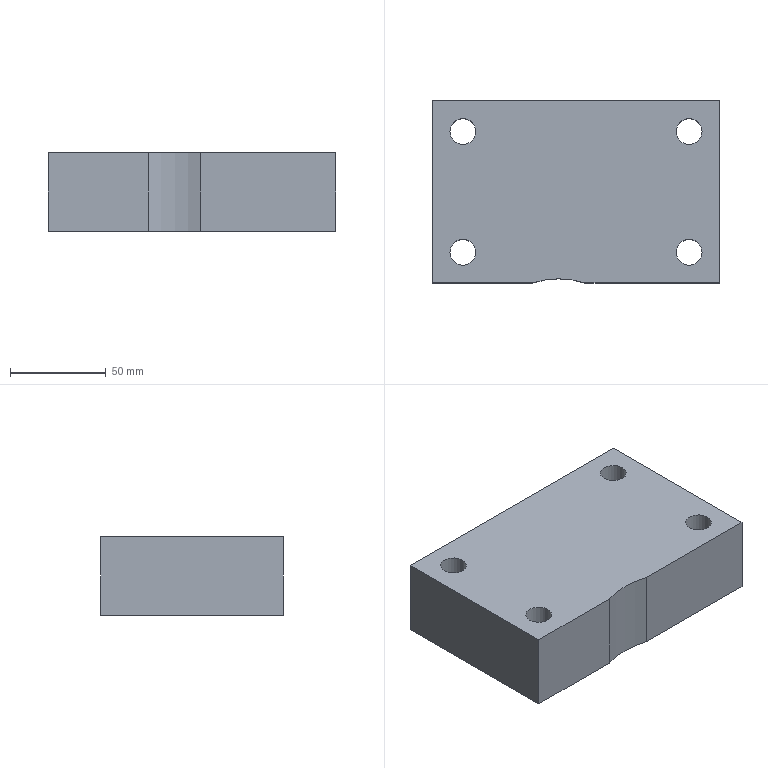Part | NX | features solid 2 | 1 solid | 20 faces | box 150 x 95 x 41 mm | volume 548863 mm3 | plane 11 | cylinder 9 | commonest cylinder face diameters 13.5 x4 20 x4 88 x1
STEP:
#1=CARTESIAN_POINT('',(1702.713,264.808,60.));
#2=VERTEX_POINT('',#1);
#3=CARTESIAN_POINT('',(1702.713,264.808,101.));
#4=VERTEX_POINT('',#3);
#5=CARTESIAN_POINT('',(1702.713,264.808,50.));
#6=DIRECTION('',(0.,0.,1.));
#7=VECTOR('',#6,1000.);
#8=LINE('',#5,#7);
#9=EDGE_CURVE('',#2,#4,#8,.T.);
#10=ORIENTED_EDGE('',*,*,#9,.F.);
#11=CARTESIAN_POINT('',(1773.045,264.808,60.));
#12=VERTEX_POINT('',#11);
#13=CARTESIAN_POINT('',(1698.045,264.808,60.));
#14=DIRECTION('',(1.,0.,0.));
#15=VECTOR('',#14,1000.);
#16=LINE('',#13,#15);
#17=EDGE_CURVE('',#2,#12,#16,.T.);
#18=ORIENTED_EDGE('',*,*,#17,.T.);
#19=CARTESIAN_POINT('',(1773.045,264.808,101.));
#20=VERTEX_POINT('',#19);
#21=CARTESIAN_POINT('',(1773.045,264.808,81.));
#22=DIRECTION('',(0.,0.,1.));
#23=VECTOR('',#22,1000.);
#24=LINE('',#21,#23);
#25=EDGE_CURVE('',#12,#20,#24,.T.);
#26=ORIENTED_EDGE('',*,*,#25,.T.);
#27=CARTESIAN_POINT('',(1698.045,264.808,101.));
#28=DIRECTION('',(-1.,0.,0.));
#29=VECTOR('',#28,1000.);
#30=LINE('',#27,#29);
#31=EDGE_CURVE('',#20,#4,#30,.T.);
#32=ORIENTED_EDGE('',*,*,#31,.T.);
#33=EDGE_LOOP('',(#10,#18,#26,#32));
#34=FACE_BOUND('',#33,.T.);
#35=CARTESIAN_POINT('',(1698.045,264.808,81.));
#36=DIRECTION('',(0.,-1.,0.));
#37=DIRECTION('',(0.,0.,1.));
#38=AXIS2_PLACEMENT_3D('',#35,#36,#37);
#39=PLANE('',#38);
#40=ADVANCED_FACE('',(#34),#39,.T.);
#41=CARTESIAN_POINT('',(1675.287,264.808,60.));
#42=VERTEX_POINT('',#41);
#43=CARTESIAN_POINT('',(1689.,223.,60.));
#44=DIRECTION('',(0.,0.,-1.));
#45=DIRECTION('',(-1.,0.,0.));
#46=AXIS2_PLACEMENT_3D('',#43,#44,#45);
#47=CIRCLE('',#46,44.);
#48=EDGE_CURVE('',#42,#2,#47,.T.);
#49=ORIENTED_EDGE('',*,*,#48,.F.);
#50=CARTESIAN_POINT('',(1623.045,264.808,60.));
#51=VERTEX_POINT('',#50);
#52=CARTESIAN_POINT('',(1698.045,264.808,60.));
#53=DIRECTION('',(1.,0.,0.));
#54=VECTOR('',#53,1000.);
#55=LINE('',#52,#54);
#56=EDGE_CURVE('',#51,#42,#55,.T.);
#57=ORIENTED_EDGE('',*,*,#56,.F.);
#58=CARTESIAN_POINT('',(1623.045,359.808,60.));
#59=VERTEX_POINT('',#58);
#60=CARTESIAN_POINT('',(1623.045,312.308,60.));
#61=DIRECTION('',(0.,-1.,0.));
#62=VECTOR('',#61,1000.);
#63=LINE('',#60,#62);
#64=EDGE_CURVE('',#59,#51,#63,.T.);
#65=ORIENTED_EDGE('',*,*,#64,.F.);
#66=CARTESIAN_POINT('',(1773.045,359.808,60.));
#67=VERTEX_POINT('',#66);
#68=CARTESIAN_POINT('',(1698.045,359.808,60.));
#69=DIRECTION('',(-1.,0.,0.));
#70=VECTOR('',#69,1000.);
#71=LINE('',#68,#70);
#72=EDGE_CURVE('',#67,#59,#71,.T.);
#73=ORIENTED_EDGE('',*,*,#72,.F.);
#74=CARTESIAN_POINT('',(1773.045,312.308,60.));
#75=DIRECTION('',(0.,1.,0.));
#76=VECTOR('',#75,1000.);
#77=LINE('',#74,#76);
#78=EDGE_CURVE('',#12,#67,#77,.T.);
#79=ORIENTED_EDGE('',*,*,#78,.F.);
#80=ORIENTED_EDGE('',*,*,#17,.F.);
#81=EDGE_LOOP('',(#49,#57,#65,#73,#79,#80));
#82=FACE_BOUND('',#81,.T.);
#83=CARTESIAN_POINT('',(1767.045,280.808,60.));
#84=VERTEX_POINT('',#83);
#85=CARTESIAN_POINT('',(1757.045,280.808,60.));
#86=DIRECTION('',(0.,0.,1.));
#87=DIRECTION('',(1.,0.,0.));
#88=AXIS2_PLACEMENT_3D('',#85,#86,#87);
#89=CIRCLE('',#88,10.);
#90=EDGE_CURVE('',#84,#84,#89,.T.);
#91=ORIENTED_EDGE('',*,*,#90,.T.);
#92=EDGE_LOOP('',(#91));
#93=FACE_BOUND('',#92,.T.);
#94=CARTESIAN_POINT('',(1649.045,343.808,60.));
#95=VERTEX_POINT('',#94);
#96=CARTESIAN_POINT('',(1639.045,343.808,60.));
#97=DIRECTION('',(0.,0.,1.));
#98=DIRECTION('',(1.,0.,0.));
#99=AXIS2_PLACEMENT_3D('',#96,#97,#98);
#100=CIRCLE('',#99,10.);
#101=EDGE_CURVE('',#95,#95,#100,.T.);
#102=ORIENTED_EDGE('',*,*,#101,.T.);
#103=EDGE_LOOP('',(#102));
#104=FACE_BOUND('',#103,.T.);
#105=CARTESIAN_POINT('',(1649.045,280.808,60.));
#106=VERTEX_POINT('',#105);
#107=CARTESIAN_POINT('',(1639.045,280.808,60.));
#108=DIRECTION('',(0.,0.,1.));
#109=DIRECTION('',(1.,0.,0.));
#110=AXIS2_PLACEMENT_3D('',#107,#108,#109);
#111=CIRCLE('',#110,10.);
#112=EDGE_CURVE('',#106,#106,#111,.T.);
#113=ORIENTED_EDGE('',*,*,#112,.T.);
#114=EDGE_LOOP('',(#113));
#115=FACE_BOUND('',#114,.T.);
#116=CARTESIAN_POINT('',(1767.045,343.808,60.));
#117=VERTEX_POINT('',#116);
#118=CARTESIAN_POINT('',(1757.045,343.808,60.));
#119=DIRECTION('',(0.,0.,1.));
#120=DIRECTION('',(1.,0.,0.));
#121=AXIS2_PLACEMENT_3D('',#118,#119,#120);
#122=CIRCLE('',#121,10.);
#123=EDGE_CURVE('',#117,#117,#122,.T.);
#124=ORIENTED_EDGE('',*,*,#123,.T.);
#125=EDGE_LOOP('',(#124));
#126=FACE_BOUND('',#125,.T.);
#127=CARTESIAN_POINT('',(1698.045,312.308,60.));
#128=DIRECTION('',(0.,0.,-1.));
#129=DIRECTION('',(1.,0.,0.));
#130=AXIS2_PLACEMENT_3D('',#127,#128,#129);
#131=PLANE('',#130);
#132=ADVANCED_FACE('',(#82,#93,#104,#115,#126),#131,.T.);
#133=CARTESIAN_POINT('',(1675.287,264.808,101.));
#134=VERTEX_POINT('',#133);
#135=CARTESIAN_POINT('',(1689.,223.,101.));
#136=DIRECTION('',(0.,0.,1.));
#137=DIRECTION('',(1.,0.,0.));
#138=AXIS2_PLACEMENT_3D('',#135,#136,#137);
#139=CIRCLE('',#138,44.);
#140=EDGE_CURVE('',#4,#134,#139,.T.);
#141=ORIENTED_EDGE('',*,*,#140,.F.);
#142=ORIENTED_EDGE('',*,*,#31,.F.);
#143=CARTESIAN_POINT('',(1773.045,359.808,101.));
#144=VERTEX_POINT('',#143);
#145=CARTESIAN_POINT('',(1773.045,312.308,101.));
#146=DIRECTION('',(0.,-1.,0.));
#147=VECTOR('',#146,1000.);
#148=LINE('',#145,#147);
#149=EDGE_CURVE('',#144,#20,#148,.T.);
#150=ORIENTED_EDGE('',*,*,#149,.F.);
#151=CARTESIAN_POINT('',(1623.045,359.808,101.));
#152=VERTEX_POINT('',#151);
#153=CARTESIAN_POINT('',(1698.045,359.808,101.));
#154=DIRECTION('',(1.,0.,0.));
#155=VECTOR('',#154,1000.);
#156=LINE('',#153,#155);
#157=EDGE_CURVE('',#152,#144,#156,.T.);
#158=ORIENTED_EDGE('',*,*,#157,.F.);
#159=CARTESIAN_POINT('',(1623.045,264.808,101.));
#160=VERTEX_POINT('',#159);
#161=CARTESIAN_POINT('',(1623.045,312.308,101.));
#162=DIRECTION('',(0.,1.,0.));
#163=VECTOR('',#162,1000.);
#164=LINE('',#161,#163);
#165=EDGE_CURVE('',#160,#152,#164,.T.);
#166=ORIENTED_EDGE('',*,*,#165,.F.);
#167=CARTESIAN_POINT('',(1698.045,264.808,101.));
#168=DIRECTION('',(-1.,0.,0.));
#169=VECTOR('',#168,1000.);
#170=LINE('',#167,#169);
#171=EDGE_CURVE('',#134,#160,#170,.T.);
#172=ORIENTED_EDGE('',*,*,#171,.F.);
#173=EDGE_LOOP('',(#141,#142,#150,#158,#166,#172));
#174=FACE_BOUND('',#173,.T.);
#175=CARTESIAN_POINT('',(1763.795,343.808,101.));
#176=VERTEX_POINT('',#175);
#177=CARTESIAN_POINT('',(1757.045,343.808,101.));
#178=DIRECTION('',(0.,0.,1.));
#179=DIRECTION('',(1.,0.,0.));
#180=AXIS2_PLACEMENT_3D('',#177,#178,#179);
#181=CIRCLE('',#180,6.75);
#182=EDGE_CURVE('',#176,#176,#181,.T.);
#183=ORIENTED_EDGE('',*,*,#182,.F.);
#184=EDGE_LOOP('',(#183));
#185=FACE_BOUND('',#184,.T.);
#186=CARTESIAN_POINT('',(1763.795,280.808,101.));
#187=VERTEX_POINT('',#186);
#188=CARTESIAN_POINT('',(1757.045,280.808,101.));
#189=DIRECTION('',(0.,0.,1.));
#190=DIRECTION('',(1.,0.,0.));
#191=AXIS2_PLACEMENT_3D('',#188,#189,#190);
#192=CIRCLE('',#191,6.75);
#193=EDGE_CURVE('',#187,#187,#192,.T.);
#194=ORIENTED_EDGE('',*,*,#193,.F.);
#195=EDGE_LOOP('',(#194));
#196=FACE_BOUND('',#195,.T.);
#197=CARTESIAN_POINT('',(1645.795,280.808,101.));
#198=VERTEX_POINT('',#197);
#199=CARTESIAN_POINT('',(1639.045,280.808,101.));
#200=DIRECTION('',(0.,0.,1.));
#201=DIRECTION('',(1.,0.,0.));
#202=AXIS2_PLACEMENT_3D('',#199,#200,#201);
#203=CIRCLE('',#202,6.75);
#204=EDGE_CURVE('',#198,#198,#203,.T.);
#205=ORIENTED_EDGE('',*,*,#204,.F.);
#206=EDGE_LOOP('',(#205));
#207=FACE_BOUND('',#206,.T.);
#208=CARTESIAN_POINT('',(1645.795,343.808,101.));
#209=VERTEX_POINT('',#208);
#210=CARTESIAN_POINT('',(1639.045,343.808,101.));
#211=DIRECTION('',(0.,0.,1.));
#212=DIRECTION('',(1.,0.,0.));
#213=AXIS2_PLACEMENT_3D('',#210,#211,#212);
#214=CIRCLE('',#213,6.75);
#215=EDGE_CURVE('',#209,#209,#214,.T.);
#216=ORIENTED_EDGE('',*,*,#215,.F.);
#217=EDGE_LOOP('',(#216));
#218=FACE_BOUND('',#217,.T.);
#219=CARTESIAN_POINT('',(1698.045,312.308,101.));
#220=DIRECTION('',(0.,0.,1.));
#221=DIRECTION('',(-1.,0.,0.));
#222=AXIS2_PLACEMENT_3D('',#219,#220,#221);
#223=PLANE('',#222);
#224=ADVANCED_FACE('',(#174,#185,#196,#207,#218),#223,.T.);
#225=CARTESIAN_POINT('',(1675.287,264.808,50.));
#226=DIRECTION('',(0.,0.,-1.));
#227=VECTOR('',#226,1000.);
#228=LINE('',#225,#227);
#229=EDGE_CURVE('',#134,#42,#228,.T.);
#230=ORIENTED_EDGE('',*,*,#229,.F.);
#231=ORIENTED_EDGE('',*,*,#171,.T.);
#232=CARTESIAN_POINT('',(1623.045,264.808,81.));
#233=DIRECTION('',(0.,0.,1.));
#234=VECTOR('',#233,1000.);
#235=LINE('',#232,#234);
#236=EDGE_CURVE('',#51,#160,#235,.T.);
#237=ORIENTED_EDGE('',*,*,#236,.F.);
#238=ORIENTED_EDGE('',*,*,#56,.T.);
#239=EDGE_LOOP('',(#230,#231,#237,#238));
#240=FACE_BOUND('',#239,.T.);
#241=CARTESIAN_POINT('',(1698.045,264.808,81.));
#242=DIRECTION('',(0.,-1.,0.));
#243=DIRECTION('',(0.,0.,1.));
#244=AXIS2_PLACEMENT_3D('',#241,#242,#243);
#245=PLANE('',#244);
#246=ADVANCED_FACE('',(#240),#245,.T.);
#247=ORIENTED_EDGE('',*,*,#236,.T.);
#248=ORIENTED_EDGE('',*,*,#165,.T.);
#249=CARTESIAN_POINT('',(1623.045,359.808,81.));
#250=DIRECTION('',(0.,0.,1.));
#251=VECTOR('',#250,1000.);
#252=LINE('',#249,#251);
#253=EDGE_CURVE('',#59,#152,#252,.T.);
#254=ORIENTED_EDGE('',*,*,#253,.F.);
#255=ORIENTED_EDGE('',*,*,#64,.T.);
#256=EDGE_LOOP('',(#247,#248,#254,#255));
#257=FACE_BOUND('',#256,.T.);
#258=CARTESIAN_POINT('',(1623.045,312.308,81.));
#259=DIRECTION('',(-1.,0.,0.));
#260=DIRECTION('',(0.,0.,-1.));
#261=AXIS2_PLACEMENT_3D('',#258,#259,#260);
#262=PLANE('',#261);
#263=ADVANCED_FACE('',(#257),#262,.T.);
#264=ORIENTED_EDGE('',*,*,#253,.T.);
#265=ORIENTED_EDGE('',*,*,#157,.T.);
#266=CARTESIAN_POINT('',(1773.045,359.808,81.));
#267=DIRECTION('',(0.,0.,1.));
#268=VECTOR('',#267,1000.);
#269=LINE('',#266,#268);
#270=EDGE_CURVE('',#67,#144,#269,.T.);
#271=ORIENTED_EDGE('',*,*,#270,.F.);
#272=ORIENTED_EDGE('',*,*,#72,.T.);
#273=EDGE_LOOP('',(#264,#265,#271,#272));
#274=FACE_BOUND('',#273,.T.);
#275=CARTESIAN_POINT('',(1698.045,359.808,81.));
#276=DIRECTION('',(0.,1.,0.));
#277=DIRECTION('',(0.,0.,-1.));
#278=AXIS2_PLACEMENT_3D('',#275,#276,#277);
#279=PLANE('',#278);
#280=ADVANCED_FACE('',(#274),#279,.T.);
#281=ORIENTED_EDGE('',*,*,#78,.T.);
#282=ORIENTED_EDGE('',*,*,#270,.T.);
#283=ORIENTED_EDGE('',*,*,#149,.T.);
#284=ORIENTED_EDGE('',*,*,#25,.F.);
#285=EDGE_LOOP('',(#281,#282,#283,#284));
#286=FACE_BOUND('',#285,.T.);
#287=CARTESIAN_POINT('',(1773.045,312.308,81.));
#288=DIRECTION('',(1.,0.,0.));
#289=DIRECTION('',(0.,0.,1.));
#290=AXIS2_PLACEMENT_3D('',#287,#288,#289);
#291=PLANE('',#290);
#292=ADVANCED_FACE('',(#286),#291,.T.);
#293=ORIENTED_EDGE('',*,*,#215,.T.);
#294=EDGE_LOOP('',(#293));
#295=FACE_BOUND('',#294,.T.);
#296=CARTESIAN_POINT('',(1645.795,343.808,75.));
#297=VERTEX_POINT('',#296);
#298=CARTESIAN_POINT('',(1639.045,343.808,75.));
#299=DIRECTION('',(0.,0.,1.));
#300=DIRECTION('',(1.,0.,0.));
#301=AXIS2_PLACEMENT_3D('',#298,#299,#300);
#302=CIRCLE('',#301,6.75);
#303=EDGE_CURVE('',#297,#297,#302,.T.);
#304=ORIENTED_EDGE('',*,*,#303,.F.);
#305=EDGE_LOOP('',(#304));
#306=FACE_BOUND('',#305,.T.);
#307=CARTESIAN_POINT('',(1639.045,343.808,55.));
#308=DIRECTION('',(0.,0.,1.));
#309=DIRECTION('',(-1.,0.,0.));
#310=AXIS2_PLACEMENT_3D('',#307,#308,#309);
#311=CYLINDRICAL_SURFACE('',#310,6.75);
#312=ADVANCED_FACE('',(#295,#306),#311,.F.);
#313=ORIENTED_EDGE('',*,*,#303,.T.);
#314=EDGE_LOOP('',(#313));
#315=FACE_BOUND('',#314,.T.);
#316=CARTESIAN_POINT('',(1649.045,343.808,75.));
#317=VERTEX_POINT('',#316);
#318=CARTESIAN_POINT('',(1639.045,343.808,75.));
#319=DIRECTION('',(0.,0.,1.));
#320=DIRECTION('',(1.,0.,0.));
#321=AXIS2_PLACEMENT_3D('',#318,#319,#320);
#322=CIRCLE('',#321,10.);
#323=EDGE_CURVE('',#317,#317,#322,.T.);
#324=ORIENTED_EDGE('',*,*,#323,.F.);
#325=EDGE_LOOP('',(#324));
#326=FACE_BOUND('',#325,.T.);
#327=CARTESIAN_POINT('',(1639.045,343.808,75.));
#328=DIRECTION('',(0.,0.,1.));
#329=DIRECTION('',(-1.,0.,0.));
#330=AXIS2_PLACEMENT_3D('',#327,#328,#329);
#331=PLANE('',#330);
#332=ADVANCED_FACE('',(#315,#326),#331,.F.);
#333=ORIENTED_EDGE('',*,*,#323,.T.);
#334=EDGE_LOOP('',(#333));
#335=FACE_BOUND('',#334,.T.);
#336=ORIENTED_EDGE('',*,*,#101,.F.);
#337=EDGE_LOOP('',(#336));
#338=FACE_BOUND('',#337,.T.);
#339=CARTESIAN_POINT('',(1639.045,343.808,60.));
#340=DIRECTION('',(0.,0.,1.));
#341=DIRECTION('',(-1.,0.,0.));
#342=AXIS2_PLACEMENT_3D('',#339,#340,#341);
#343=CYLINDRICAL_SURFACE('',#342,10.);
#344=ADVANCED_FACE('',(#335,#338),#343,.F.);
#345=ORIENTED_EDGE('',*,*,#204,.T.);
#346=EDGE_LOOP('',(#345));
#347=FACE_BOUND('',#346,.T.);
#348=CARTESIAN_POINT('',(1645.795,280.808,75.));
#349=VERTEX_POINT('',#348);
#350=CARTESIAN_POINT('',(1639.045,280.808,75.));
#351=DIRECTION('',(0.,0.,1.));
#352=DIRECTION('',(1.,0.,0.));
#353=AXIS2_PLACEMENT_3D('',#350,#351,#352);
#354=CIRCLE('',#353,6.75);
#355=EDGE_CURVE('',#349,#349,#354,.T.);
#356=ORIENTED_EDGE('',*,*,#355,.F.);
#357=EDGE_LOOP('',(#356));
#358=FACE_BOUND('',#357,.T.);
#359=CARTESIAN_POINT('',(1639.045,280.808,55.));
#360=DIRECTION('',(0.,0.,1.));
#361=DIRECTION('',(-1.,0.,0.));
#362=AXIS2_PLACEMENT_3D('',#359,#360,#361);
#363=CYLINDRICAL_SURFACE('',#362,6.75);
#364=ADVANCED_FACE('',(#347,#358),#363,.F.);
#365=ORIENTED_EDGE('',*,*,#355,.T.);
#366=EDGE_LOOP('',(#365));
#367=FACE_BOUND('',#366,.T.);
#368=CARTESIAN_POINT('',(1649.045,280.808,75.));
#369=VERTEX_POINT('',#368);
#370=CARTESIAN_POINT('',(1639.045,280.808,75.));
#371=DIRECTION('',(0.,0.,1.));
#372=DIRECTION('',(1.,0.,0.));
#373=AXIS2_PLACEMENT_3D('',#370,#371,#372);
#374=CIRCLE('',#373,10.);
#375=EDGE_CURVE('',#369,#369,#374,.T.);
#376=ORIENTED_EDGE('',*,*,#375,.F.);
#377=EDGE_LOOP('',(#376));
#378=FACE_BOUND('',#377,.T.);
#379=CARTESIAN_POINT('',(1639.045,280.808,75.));
#380=DIRECTION('',(0.,0.,1.));
#381=DIRECTION('',(-1.,0.,0.));
#382=AXIS2_PLACEMENT_3D('',#379,#380,#381);
#383=PLANE('',#382);
#384=ADVANCED_FACE('',(#367,#378),#383,.F.);
#385=ORIENTED_EDGE('',*,*,#375,.T.);
#386=EDGE_LOOP('',(#385));
#387=FACE_BOUND('',#386,.T.);
#388=ORIENTED_EDGE('',*,*,#112,.F.);
#389=EDGE_LOOP('',(#388));
#390=FACE_BOUND('',#389,.T.);
#391=CARTESIAN_POINT('',(1639.045,280.808,60.));
#392=DIRECTION('',(0.,0.,1.));
#393=DIRECTION('',(-1.,0.,0.));
#394=AXIS2_PLACEMENT_3D('',#391,#392,#393);
#395=CYLINDRICAL_SURFACE('',#394,10.);
#396=ADVANCED_FACE('',(#387,#390),#395,.F.);
#397=ORIENTED_EDGE('',*,*,#193,.T.);
#398=EDGE_LOOP('',(#397));
#399=FACE_BOUND('',#398,.T.);
#400=CARTESIAN_POINT('',(1763.795,280.808,75.));
#401=VERTEX_POINT('',#400);
#402=CARTESIAN_POINT('',(1757.045,280.808,75.));
#403=DIRECTION('',(0.,0.,1.));
#404=DIRECTION('',(1.,0.,0.));
#405=AXIS2_PLACEMENT_3D('',#402,#403,#404);
#406=CIRCLE('',#405,6.75);
#407=EDGE_CURVE('',#401,#401,#406,.T.);
#408=ORIENTED_EDGE('',*,*,#407,.F.);
#409=EDGE_LOOP('',(#408));
#410=FACE_BOUND('',#409,.T.);
#411=CARTESIAN_POINT('',(1757.045,280.808,55.));
#412=DIRECTION('',(0.,0.,1.));
#413=DIRECTION('',(-1.,0.,0.));
#414=AXIS2_PLACEMENT_3D('',#411,#412,#413);
#415=CYLINDRICAL_SURFACE('',#414,6.75);
#416=ADVANCED_FACE('',(#399,#410),#415,.F.);
#417=ORIENTED_EDGE('',*,*,#407,.T.);
#418=EDGE_LOOP('',(#417));
#419=FACE_BOUND('',#418,.T.);
#420=CARTESIAN_POINT('',(1767.045,280.808,75.));
#421=VERTEX_POINT('',#420);
#422=CARTESIAN_POINT('',(1757.045,280.808,75.));
#423=DIRECTION('',(0.,0.,1.));
#424=DIRECTION('',(1.,0.,0.));
#425=AXIS2_PLACEMENT_3D('',#422,#423,#424);
#426=CIRCLE('',#425,10.);
#427=EDGE_CURVE('',#421,#421,#426,.T.);
#428=ORIENTED_EDGE('',*,*,#427,.F.);
#429=EDGE_LOOP('',(#428));
#430=FACE_BOUND('',#429,.T.);
#431=CARTESIAN_POINT('',(1757.045,280.808,75.));
#432=DIRECTION('',(0.,0.,1.));
#433=DIRECTION('',(-1.,0.,0.));
#434=AXIS2_PLACEMENT_3D('',#431,#432,#433);
#435=PLANE('',#434);
#436=ADVANCED_FACE('',(#419,#430),#435,.F.);
#437=ORIENTED_EDGE('',*,*,#427,.T.);
#438=EDGE_LOOP('',(#437));
#439=FACE_BOUND('',#438,.T.);
#440=ORIENTED_EDGE('',*,*,#90,.F.);
#441=EDGE_LOOP('',(#440));
#442=FACE_BOUND('',#441,.T.);
#443=CARTESIAN_POINT('',(1757.045,280.808,60.));
#444=DIRECTION('',(0.,0.,1.));
#445=DIRECTION('',(-1.,0.,0.));
#446=AXIS2_PLACEMENT_3D('',#443,#444,#445);
#447=CYLINDRICAL_SURFACE('',#446,10.);
#448=ADVANCED_FACE('',(#439,#442),#447,.F.);
#449=ORIENTED_EDGE('',*,*,#182,.T.);
#450=EDGE_LOOP('',(#449));
#451=FACE_BOUND('',#450,.T.);
#452=CARTESIAN_POINT('',(1763.795,343.808,75.));
#453=VERTEX_POINT('',#452);
#454=CARTESIAN_POINT('',(1757.045,343.808,75.));
#455=DIRECTION('',(0.,0.,1.));
#456=DIRECTION('',(1.,0.,0.));
#457=AXIS2_PLACEMENT_3D('',#454,#455,#456);
#458=CIRCLE('',#457,6.75);
#459=EDGE_CURVE('',#453,#453,#458,.T.);
#460=ORIENTED_EDGE('',*,*,#459,.F.);
#461=EDGE_LOOP('',(#460));
#462=FACE_BOUND('',#461,.T.);
#463=CARTESIAN_POINT('',(1757.045,343.808,55.));
#464=DIRECTION('',(0.,0.,1.));
#465=DIRECTION('',(-1.,0.,0.));
#466=AXIS2_PLACEMENT_3D('',#463,#464,#465);
#467=CYLINDRICAL_SURFACE('',#466,6.75);
#468=ADVANCED_FACE('',(#451,#462),#467,.F.);
#469=ORIENTED_EDGE('',*,*,#459,.T.);
#470=EDGE_LOOP('',(#469));
#471=FACE_BOUND('',#470,.T.);
#472=CARTESIAN_POINT('',(1767.045,343.808,75.));
#473=VERTEX_POINT('',#472);
#474=CARTESIAN_POINT('',(1757.045,343.808,75.));
#475=DIRECTION('',(0.,0.,1.));
#476=DIRECTION('',(1.,0.,0.));
#477=AXIS2_PLACEMENT_3D('',#474,#475,#476);
#478=CIRCLE('',#477,10.);
#479=EDGE_CURVE('',#473,#473,#478,.T.);
#480=ORIENTED_EDGE('',*,*,#479,.F.);
#481=EDGE_LOOP('',(#480));
#482=FACE_BOUND('',#481,.T.);
#483=CARTESIAN_POINT('',(1757.045,343.808,75.));
#484=DIRECTION('',(0.,0.,1.));
#485=DIRECTION('',(-1.,0.,0.));
#486=AXIS2_PLACEMENT_3D('',#483,#484,#485);
#487=PLANE('',#486);
#488=ADVANCED_FACE('',(#471,#482),#487,.F.);
#489=ORIENTED_EDGE('',*,*,#479,.T.);
#490=EDGE_LOOP('',(#489));
#491=FACE_BOUND('',#490,.T.);
#492=ORIENTED_EDGE('',*,*,#123,.F.);
#493=EDGE_LOOP('',(#492));
#494=FACE_BOUND('',#493,.T.);
#495=CARTESIAN_POINT('',(1757.045,343.808,60.));
#496=DIRECTION('',(0.,0.,1.));
#497=DIRECTION('',(-1.,0.,0.));
#498=AXIS2_PLACEMENT_3D('',#495,#496,#497);
#499=CYLINDRICAL_SURFACE('',#498,10.);
#500=ADVANCED_FACE('',(#491,#494),#499,.F.);
#501=ORIENTED_EDGE('',*,*,#9,.T.);
#502=ORIENTED_EDGE('',*,*,#140,.T.);
#503=ORIENTED_EDGE('',*,*,#229,.T.);
#504=ORIENTED_EDGE('',*,*,#48,.T.);
#505=EDGE_LOOP('',(#501,#502,#503,#504));
#506=FACE_BOUND('',#505,.T.);
#507=CARTESIAN_POINT('',(1689.,223.,50.));
#508=DIRECTION('',(0.,0.,1.));
#509=DIRECTION('',(-1.,0.,0.));
#510=AXIS2_PLACEMENT_3D('',#507,#508,#509);
#511=CYLINDRICAL_SURFACE('',#510,44.);
#512=ADVANCED_FACE('',(#506),#511,.F.);
#513=CLOSED_SHELL('',(#40,#132,#224,#246,#263,#280,#292,#312,#332,#344,#364,#384,#396,#416,#436,#448,#468,#488,#500,#512));
#514=MANIFOLD_SOLID_BREP('',#513);
#515=(LENGTH_UNIT()NAMED_UNIT(*)SI_UNIT(.MILLI.,.METRE.));
#516=UNCERTAINTY_MEASURE_WITH_UNIT(LENGTH_MEASURE(0.00001),#515,'','');
#517=(NAMED_UNIT(*)PLANE_ANGLE_UNIT()SI_UNIT($,.RADIAN.));
#518=(NAMED_UNIT(*)SI_UNIT($,.STERADIAN.)SOLID_ANGLE_UNIT());
#519=(GEOMETRIC_REPRESENTATION_CONTEXT(3)GLOBAL_UNCERTAINTY_ASSIGNED_CONTEXT((#516))GLOBAL_UNIT_ASSIGNED_CONTEXT((#515,#517,#518))REPRESENTATION_CONTEXT('',''));
#520=ADVANCED_BREP_SHAPE_REPRESENTATION('',(#514),#519);